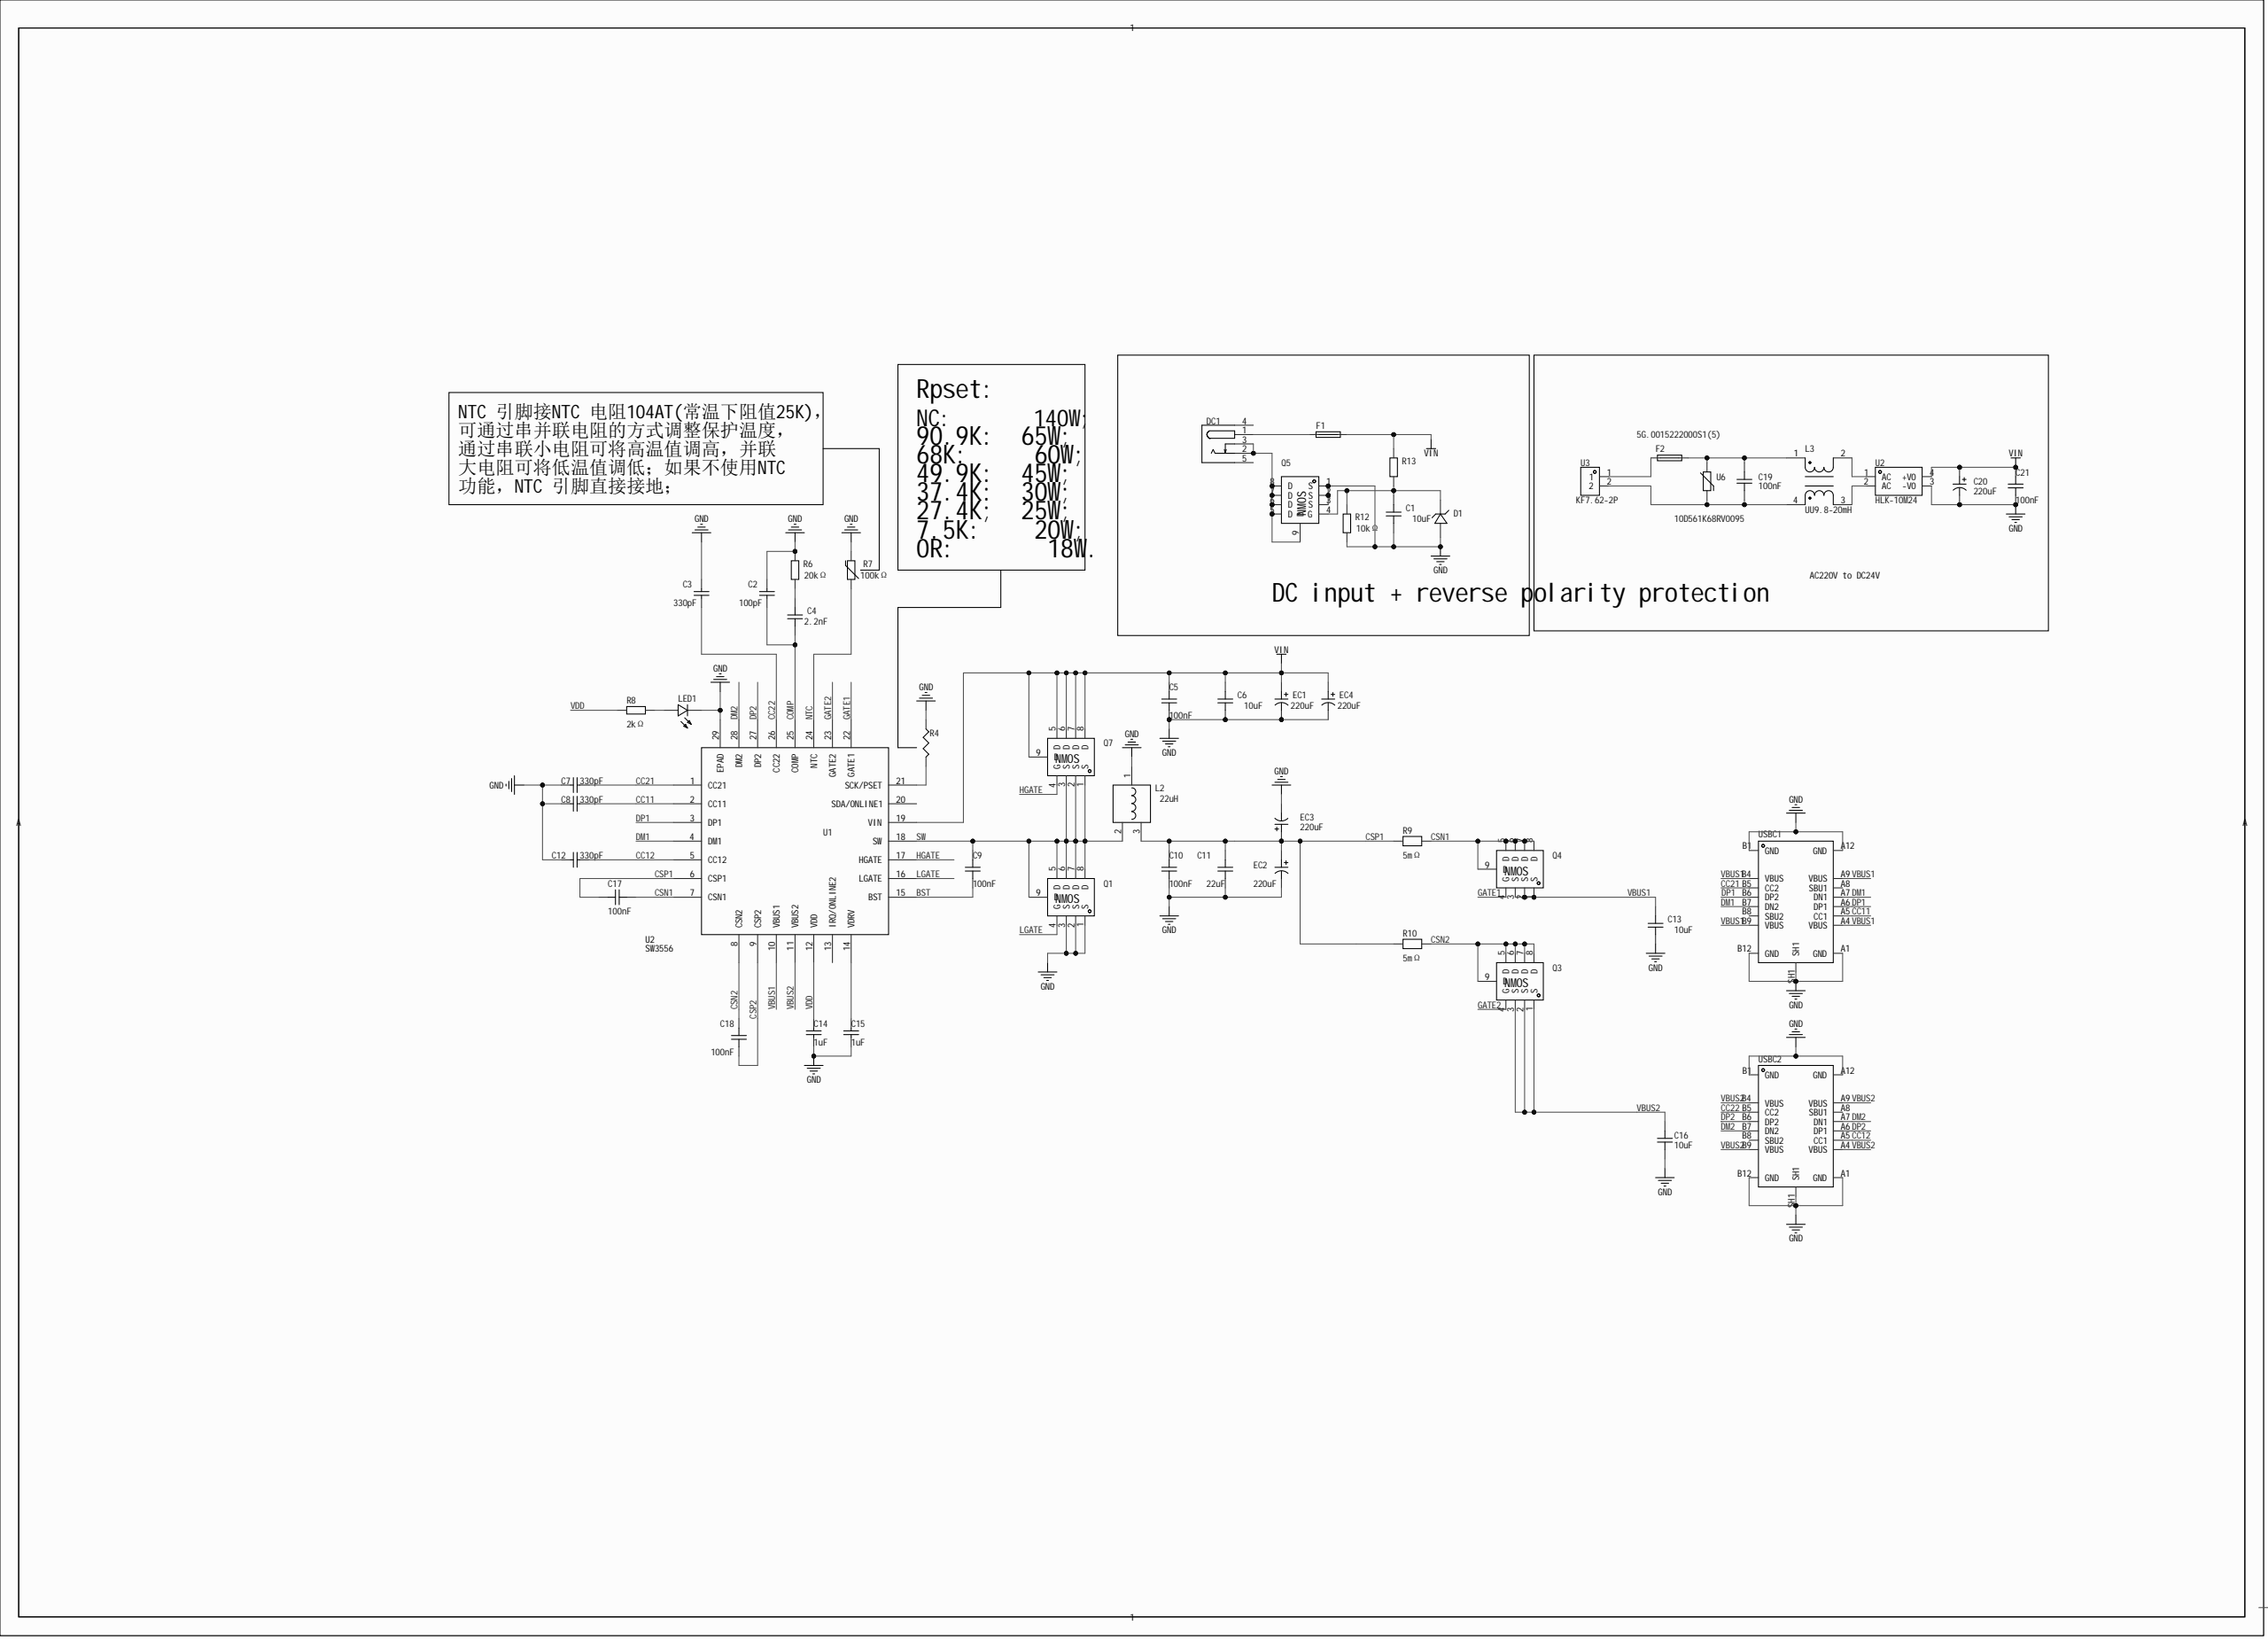Circuit board | Altium Designer | 51 parts | 36 nets
Bill of materials:
Comment,Description,Designator,Footprint,LibRef,Quantity
"10uF","Capacitance: 10uF; tolerance: ±10%; rated voltage: 50V; dielectric (temperature coefficient): X5R;","C1, C6, C13, C16","C0805","10uF","4"
"100pF","Capacitance: 100pF; tolerance: ±5%; rated voltage: 50V; dielectric (temperature coefficient): C0G;","C2","C0603","100pF","1"
"330pF","Capacitance: 330pF; tolerance: ±5%; rated voltage: 50V; dielectric (temperature coefficient): C0G;","C3, C7, C8, C12","C0603","330pF","4"
"2.2nF","Capacitance: 2.2nF; tolerance: ±1%; rated voltage: -; dielectric (temperature coefficient): -;","C4","C0603","2.2nF","1"
"100nF","Capacitance: 100nF; tolerance: ±10%; rated voltage: 50V; dielectric (temperature coefficient): X7R;","C5, C9, C10, C17, C18, C21","C0603","100nF","6"
"22uF","Capacitance: 22uF; tolerance: ±20%; rated voltage: 25V; dielectric (temperature coefficient): X5R;","C11","C0805","22uF","1"
"1uF","Capacitance: 1uF; tolerance: ±10%; rated voltage: 50V; dielectric (temperature coefficient): X5R;","C14, C15","C0603","1uF","2"
"100nF","","C19","CAP-TH_L13.0-W6.0-P10.0-D0.6","X2-104K-275VAC_C914483","1"
"220uF","","C20","CAP-TH_BD8.0-P3.50-D0.6-FD","01EC3470","1"
"BZT52C3V3","Diode configuration: single; zener voltage (nominal): 3.3V; zener voltage (range): 3.1V~3.5V; tolerance: ±5%; power: 500mW; reverse current (Ir): 20uA@1V; impedance (Zzt): 130Ω;","D1","SOD-123_L2.7-W1.6-LS3.7-RD","BZT52C3V3","1"
"DC-044A-20A","Contact inner diameter: 2mm; contact outer diameter: 5.9mm; rated current: 500mA; rated voltage: 30V;","DC1","DC-IN-TH_DC-044A-20A","DC-044A-20A","1"
"220uF","","EC1, EC2, EC3, EC4","CAP-TH_BD8.0-P3.50-D0.6-FD-2","220uF","4"
"0451008.MRL","Type: SMD fuse; rated current: 8A; rated voltage (AC): 125V; rated voltage (DC): 125V; breaking capacity: 50A; operating temperature: -55℃~+125℃;","F1","FUSE-SMD_L6.1-W2.7","0451008.MRL","1"
"5G0.001522S1(5)","","F2","FUSE-TH_BD5.6-L21.0-P25.00-D0.7","5G0.001522S1(5)","1"
"22uH","Inductance: 22uH; tolerance: ±20%; rated current: 7.5A; DC resistance (DCR): 14.5mΩ;","L2","IND-SMD_3P-L15.5-W15.5-L","22uH","1"
"UU9.8-20mH","","L3","FILTER-TH_4P-L17.0-W12.0-P7.00-D0.6-S8.00","UU9.8-20mH","1"
"19-217/BHC-ZL1M2RY/3T","Illumination color: blue; dominant wavelength / chromaticity: 465~475nm;","LED1","LED0603-R-RD","19-217/BHC-ZL1M2RY/3T","1"
"RUH4040M2","类型:-;漏源电压(Vdss):-;连续漏极电流(Id):-;功率(Pd):-;导通电阻(RDS(on)@Vgs,Id):-;阈值电压(Vgs(th)@Id):-;栅极电荷(Qg@Vgs):-;输入电容(Ciss@Vds):-;反向传输电容(Crss@Vds):-;","Q1, Q3, Q4, Q5, Q7","PDFN3333-8_L3.1-W3.2-P0.65-LS3.4-BL","RUH4040M2","5"
"Rpset","Resistor","R4","R0603","Rpset","1"
"20kΩ","","R6","R0603","20kΩ","1"
"SDNT1608X104F4250FTF","","R7","R0603","SDNT1608X104F4250FTF","1"
"0603WAF2001T5E","","R8","R0603","0603WAF2001T5E","1"
"RLM20FECR005","Resistor type: sense resistor; rated current: -; rated voltage drop: -; resistance: 5mΩ; tolerance: ±1%; power: 1W; temperature coefficient: ±50ppm/?; mounting: SMD;","R9, R10","R2010","RLM20FECR005","2"
"10kΩ","","R12","R0603","10kΩ","1"
"0603WAF5102T5E","","R13","R0603","0603WAF5102T5E","1"
"sw3556-1","","U1","QFN-28_L4.0-W4.0-P0.40-BL-EP","sw3556-1","1"
"HLK-10M24","","U2","PWRM-TH_HLK-10M24","HLK-10M24","1"
"KF7.62-2P","","U3","CONN-TH_KF7.62-2P","KF7.62-2P","1"
"10D561K68RV0095","","U6","RES-TH_L13.5-W7.0-P7.50-S4.00-D0.7","10D561K68RV0095","1"
"U263-163N-4OS1735","连接器类型:Type-C;标准:USB 3.1;公母:母座;触点数量:16;端口数量:1;安装方式:卧贴;额定电流 - 电源:5A;触头材质:铜合金;触头镀层:金;工作温度范围:-25℃~+85℃;焊接温度(最大值):260℃;","USBC1, USBC2","USB-C-SMD_U263-163N-4GS1735","U263-163N-4OS1735","2"
Netlist (Protel format):
[
C1
C0805
10uF



]
[
C2
C0603
100pF



]
[
C3
C0603
330pF



]
[
C4
C0603
2.2nF



]
[
C5
C0603
100nF



]
[
C6
C0805
10uF



]
[
C7
C0603
330pF



]
[
C8
C0603
330pF



]
[
C9
C0603
100nF



]
[
C10
C0603
100nF



]
[
C11
C0805
22uF



]
[
C12
C0603
330pF



]
[
C13
C0805
10uF



]
[
C14
C0603
1uF



]
[
C15
C0603
1uF



]
[
C16
C0805
10uF



]
[
C17
C0603
100nF



]
[
C18
C0603
100nF



]
[
C19
CAP-TH_L13.0-W6.0-P10.0-D0.6
100nF



]
[
C20
CAP-TH_BD8.0-P3.50-D0.6-FD
220uF



]
[
C21
C0603
100nF



]
[
D1
SOD-123_L2.7-W1.6-LS3.7-RD
BZT52C3V3



]
[
DC1
DC-IN-TH_DC-044A-20A
DC-044A-20A



]
[
EC1
CAP-TH_BD8.0-P3.50-D0.6-FD-2
220uF



]
[
EC2
CAP-TH_BD8.0-P3.50-D0.6-FD-2
220uF



]
[
EC3
CAP-TH_BD8.0-P3.50-D0.6-FD-2
220uF



]
[
EC4
CAP-TH_BD8.0-P3.50-D0.6-FD-2
220uF



]
[
F1
FUSE-SMD_L6.1-W2.7
0451008.MRL



]
[
F2
FUSE-TH_BD5.6-L21.0-P25.00-D0.7
5G.0015222000S1(5)



]
[
L2
IND-SMD_3P-L15.5-W15.5-L
22uH



]
[
L3
FILTER-TH_4P-L17.0-W12.0-P7.00-D0.6-S8.00
UU9.8-20mH



]
[
LED1
LED0603-R-RD
19-217/BHC-ZL1M2RY/3T



]
[
Q1
PDFN3333-8_L3.1-W3.2-P0.65-LS3.4-BL
RUH4040M2



]
[
Q3
PDFN3333-8_L3.1-W3.2-P0.65-LS3.4-BL
RUH4040M2



]
[
Q4
PDFN3333-8_L3.1-W3.2-P0.65-LS3.4-BL
RUH4040M2



]
[
Q5
PDFN3333-8_L3.1-W3.2-P0.65-LS3.4-BL
RUH4040M2



]
[
Q7
PDFN3333-8_L3.1-W3.2-P0.65-LS3.4-BL
RUH4040M2



]
[
R4
R0603
Rpset



]
[
R6
R0603
20kΩ



]
[
R7
R0603
SDNT1608X104F4250FTF



]
[
R8
R0603
0603WAF2001T5E



]
[
R9
R2010
RLM20FECR005



]
[
R10
R2010
RLM20FECR005



]
[
R12
R0603
10kΩ



]
[
R13
R0603
0603WAF5102T5E



]
[
U1
QFN-28_L4.0-W4.0-P0.40-BL-EP
sw3556-1



]
[
U2
PWRM-TH_HLK-10M24
HLK-10M24



]
[
U3
CONN-TH_KF7.62-2P
KF7.62-2P



]
[
U6
RES-TH_L13.5-W7.0-P7.50-S4.00-D0.7
10D561K68RV0095



]
[
USBC1
USB-C-SMD_U263-163N-4GS1735
U263-163N-4OS1735



]
[
USBC2
USB-C-SMD_U263-163N-4GS1735
U263-163N-4OS1735



]
(
VIN
C5-1
C6-2
C20-1
C21-1
EC1-1
EC4-1
F1-2
Q7-5
Q7-6
Q7-7
Q7-8
Q7-9
R13-2
U1-19
U2-4
)
(
VDD
C14-2
R8-1
U1-12
)
(
VBUS2
C16-2
Q3-1
Q3-2
Q3-3
U1-11
USBC2-A4
USBC2-A9
USBC2-B4
USBC2-B9
)
(
VBUS1
C13-2
Q4-1
Q4-2
Q4-3
U1-10
USBC1-A4
USBC1-A9
USBC1-B4
USBC1-B9
)
(
SW
C9-1
L2-2
Q1-5
Q1-6
Q1-7
Q1-8
Q1-9
Q7-1
Q7-2
Q7-3
U1-18
)
(
NTC
R7-2
U1-24
)
(
NetR4_2
R4-2
U1-21
)
(
NetLED1_1
LED1-1
R8-2
)
(
NetL3_3
L3-3
U2-2
)
(
NetL3_2
L3-2
U2-1
)
(
NetF2_1
F2-1
U3-1
)
(
NetDC1_2
DC1-2
DC1-3
Q5-5
Q5-6
Q5-7
Q5-8
Q5-9
)
(
NetDC1_1
DC1-1
F1-1
)
(
NetC19_2
C19-2
F2-2
L3-1
U6-2
)
(
NetC19_1
C19-1
L3-4
U3-2
U6-1
)
(
NetC15_2
C15-2
U1-14
)
(
NetC4_2
C4-2
R6-1
)
(
NetC1_2
C1-2
D1-1
Q5-4
R12-2
R13-1
)
(
LGATE
Q1-4
U1-16
)
(
HGATE
Q7-4
U1-17
)
(
GND
C1-1
C2-2
C3-2
C5-2
C6-1
C7-2
C8-2
C10-2
C11-1
C12-2
C13-1
C14-1
C15-1
C16-1
C20-2
C21-2
D1-2
EC1-2
EC2-2
EC3-2
EC4-2
L2-1
LED1-2
Q1-1
Q1-2
Q1-3
Q5-1
Q5-2
Q5-3
R4-1
R6-2
R7-1
R12-1
U1-29
U2-3
USBC1-A1
USBC1-A12
USBC1-B1
USBC1-B12
USBC1-SH1
USBC2-A1
USBC2-A12
USBC2-B1
USBC2-B12
USBC2-SH1
)
(
GATE2
Q3-4
U1-23
)
(
GATE1
Q4-4
U1-22
)
(
DP2
U1-27
USBC2-A6
USBC2-B6
)
(
DP1
U1-3
USBC1-A6
USBC1-B6
)
(
DM2
U1-28
USBC2-A7
USBC2-B7
)
(
DM1
U1-4
USBC1-A7
USBC1-B7
)
(
CSP1
C10-1
C11-2
C17-2
C18-2
EC2-1
EC3-1
L2-3
R9-1
R10-1
U1-6
U1-9
)
(
CSN2
C18-1
Q3-5
Q3-6
Q3-7
Q3-8
Q3-9
R10-2
U1-8
)
(
CSN1
C17-1
Q4-5
Q4-6
Q4-7
Q4-8
Q4-9
R9-2
U1-7
)
(
COMP
C2-1
C4-1
U1-25
)
(
CC22
C3-1
U1-26
USBC2-B5
)
(
CC21
C7-1
U1-1
USBC1-B5
)
(
CC12
C12-1
U1-5
USBC2-A5
)
(
CC11
C8-1
U1-2
USBC1-A5
)
(
BST
C9-2
U1-15
)